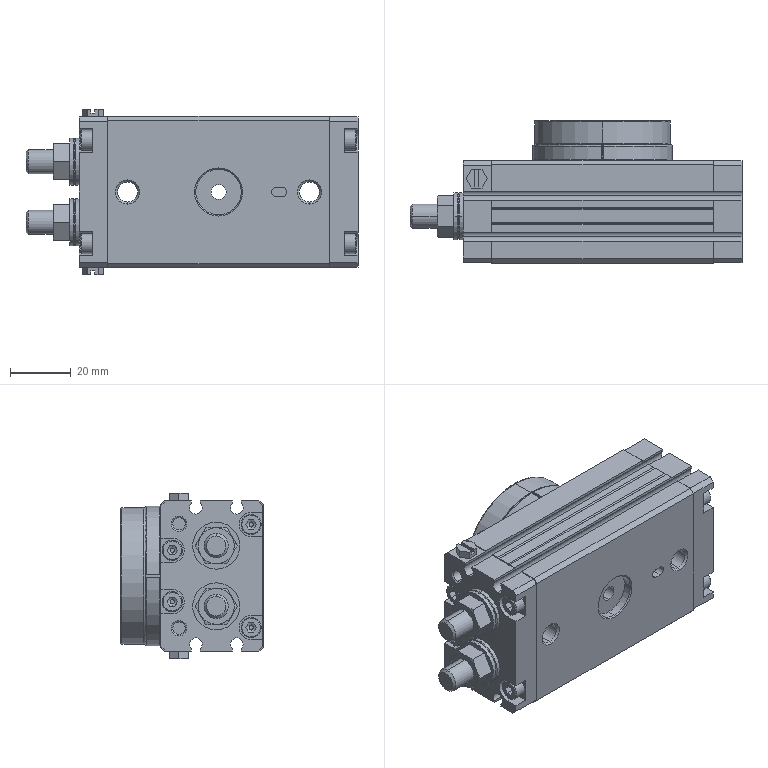Part | STEP file | HRQ10-H-2-H-21 | 1 solid | 589 faces | box 109.5 x 47 x 54.5 mm | volume 164782 mm3 | plane 309 | cylinder 133 | cone 129 | spline 18 | commonest cylinder face diameters 4.134 x28 6.66 x16 5 x14 5.5 x12 8 x12 3 x8